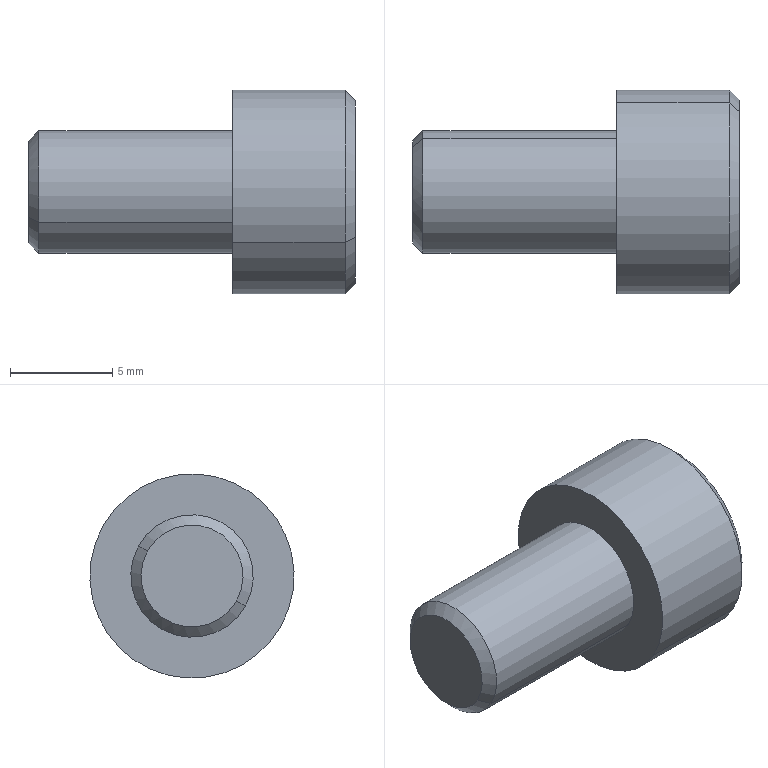Part | STEP file | Bolt M6(M6[10]) | 1 solid | 25 faces | box 16 x 10 x 10 mm | volume 667.21 mm3 | plane 15 | cone 6 | cylinder 4 | commonest cylinder face diameters 6 x2 10 x2